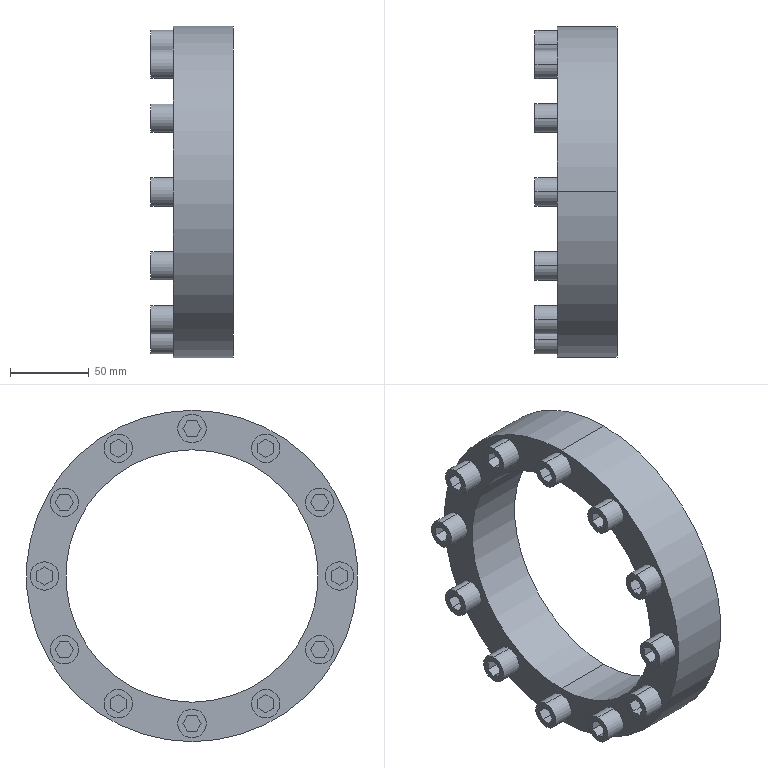Part | SolidWorks | features CirPattern 1, ICE 1, Revolution 1 | 1 solid | 126 faces | box 52 x 210 x 210 mm | volume 580630 mm3 | plane 98 | cylinder 28 | commonest cylinder face diameters 18 x24 160 x2 210 x2